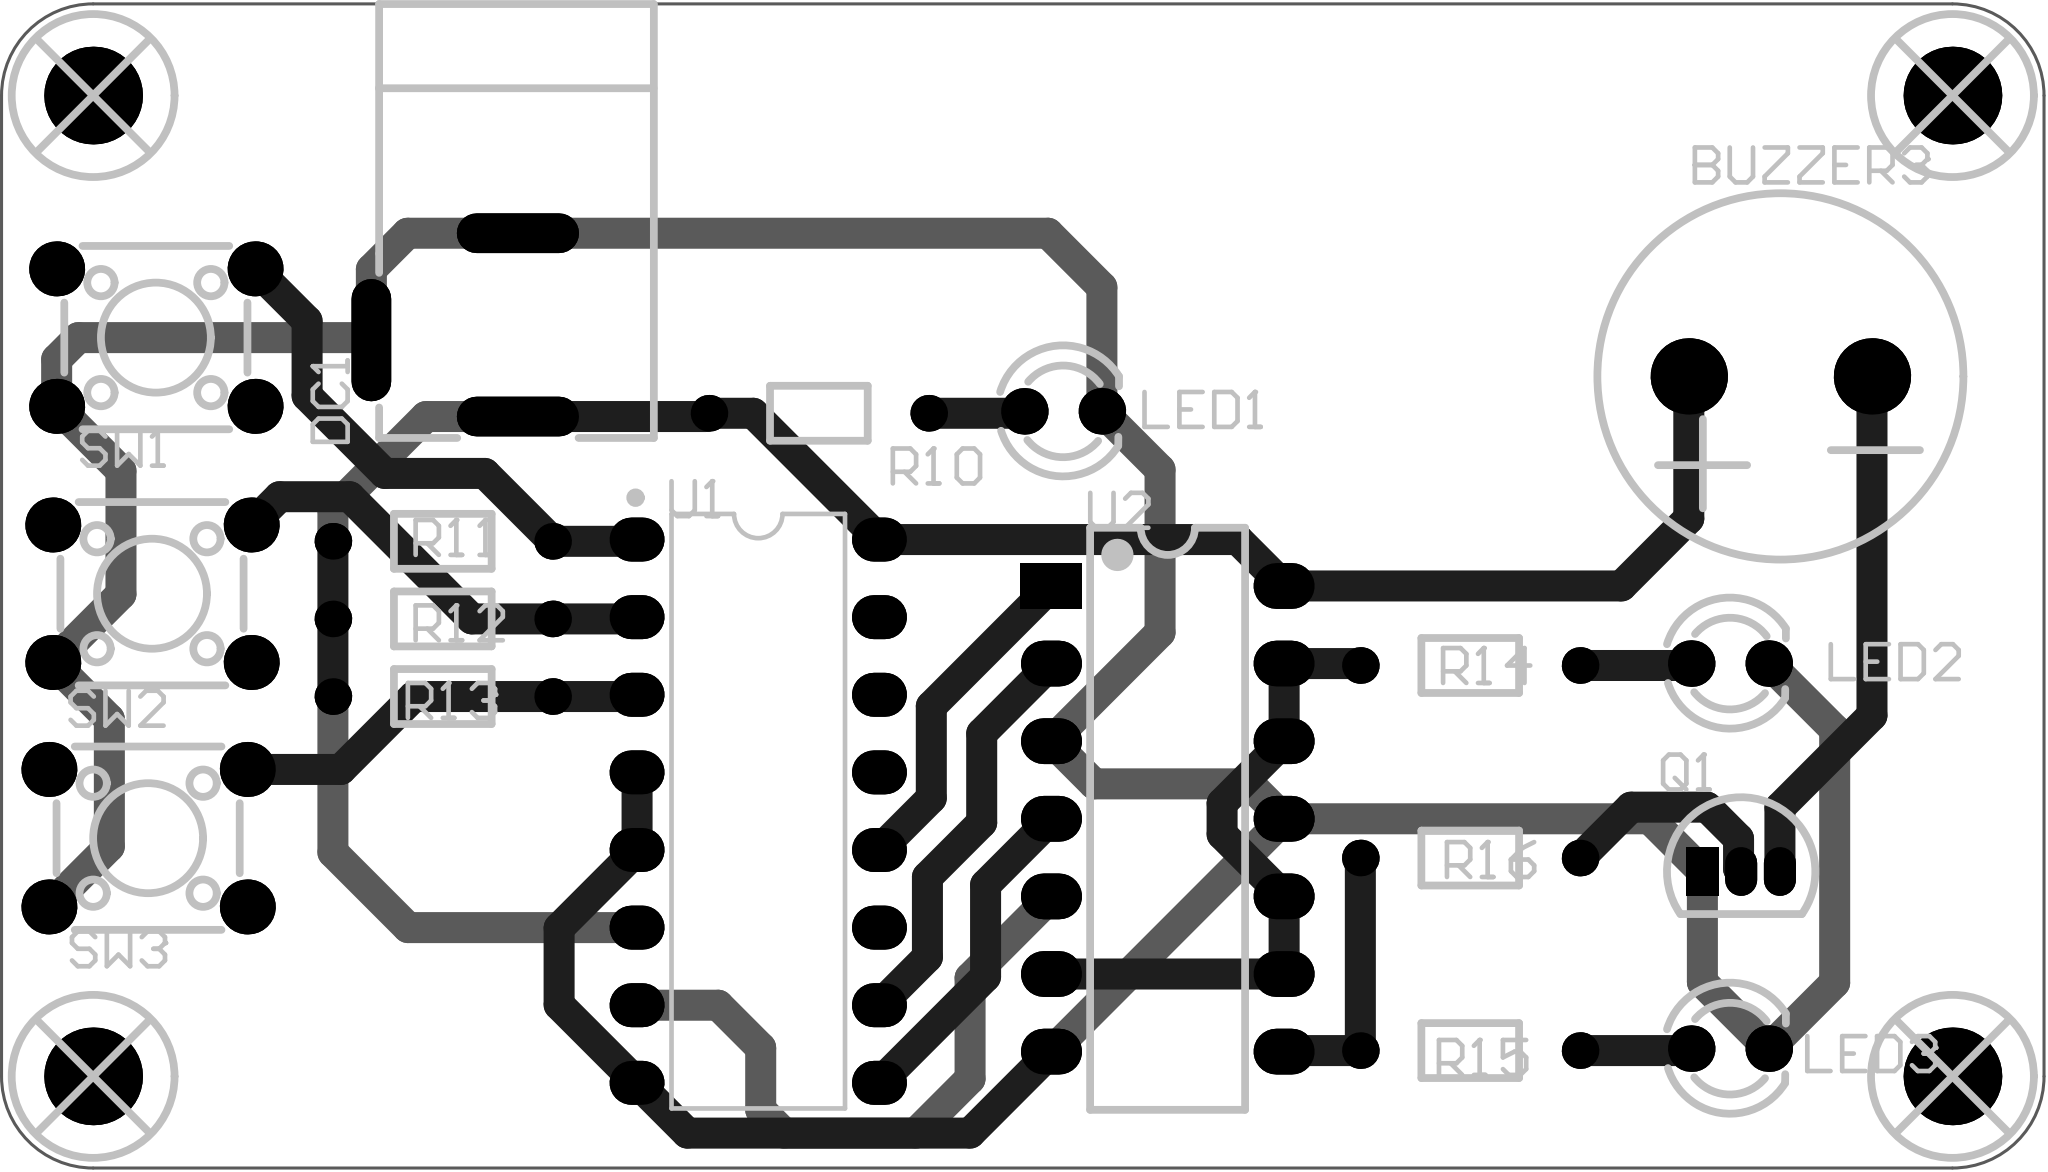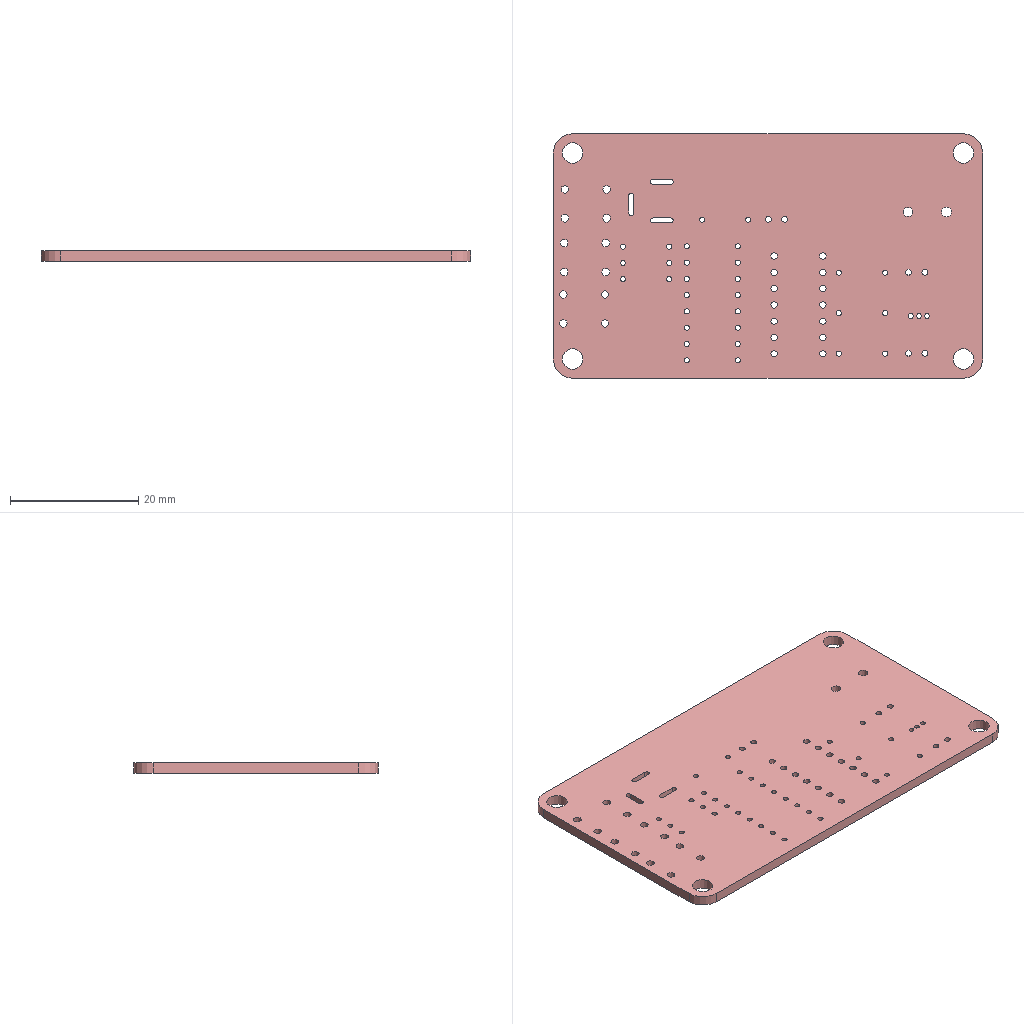Circuit board layout | Altium Designer | box 66.9 x 38.1 x 1.6 mm
Layer stack:
# Altium Designer layer stack of  (unit mm; dielectric type: 0 none, 1 core, 2 prepreg, 3 surface material)
index,name,kind,layer,copper_thickness_mm,dielectric_type,dielectric_thickness_mm,dielectric_material,dielectric_constant
0,Top Paste Mask Layer,other,,,,,,
1,Top Silkscreen Layer,other,,,,,,
2,Top Solder Mask Layer,dielectric,,,3,0.01,,3.3
3,Top Layer,copper,Top Layer,0.035,,,,
4,Dielectric1,dielectric,,,3,1.51,FR4,4.5
5,Bottom Layer,copper,Bottom Layer,0.035,,,,
6,Bottom Solder Mask Layer,dielectric,,,3,0.01,,3.3
7,Bottom Silkscreen Layer,other,,,,,,
8,Bottom Paste Mask Layer,other,,,,,,
# drill layer pairs: low layer,high layer
drill_pair,Top Layer,Bottom Layer
Part placement:
Designator,Comment,Layer,Footprint,Center-X(mm),Center-Y(mm),Rotation
LED2,,TopLayer,LED_TH-3mm,132.817,92.71,0
LED3,,TopLayer,LED_TH-3mm,132.817,80.107,0
Q1,SS8050BBU,TopLayer,TO-92-3_L4.8-W3.7-P1.27-L-1,133.183,85.905,0
SCREW1,,TopLayer,M3螺丝,79.2,79.2,0
SCREW2,,TopLayer,M3螺丝,140.104,79.2,0
SCREW3,,TopLayer,M3螺丝,79.2,111.3,0
SCREW4,,TopLayer,M3螺丝,140.104,111.3,0
R11,10kΩ,TopLayer,Res_1/8W,90.653,96.711,180
R12,10kΩ,TopLayer,Res_1/8W,90.653,94.171,180
R13,10kΩ,TopLayer,Res_1/8W,90.653,91.631,180
R14,510Ω,TopLayer,Res_1/8W,124.308,92.647,180
R15,510Ω,TopLayer,Res_1/8W,124.308,80.044,180
SW1,,TopLayer,SW-TH_4P-L6.0-W6.0-P4.50-LS6.5,81.255,103.378,180
SW2,,TopLayer,SW-TH_4P-L6.0-W6.0-P4.50-LS6.5,81.128,94.996,180
LED1,,TopLayer,LED_TH-3mm,110.973,100.965,0
R10,1kΩ,TopLayer,Res_1/8W,102.972,100.902,180
SW3,,TopLayer,SW-TH_4P-L6.0-W6.0-P4.50-LS6.5,81.001,86.995,180
U1,SN74HC138N(LX),TopLayer,PDIP-16_L19.3-W6.4-P2.54-LS7.94-BL,100.987,87.879,270
U2,SN74HC20N(LX),TopLayer,PDIP-14_L19.3-W6.5-P2.54-LS7.6-BL,114.402,87.63,270
BUZZER3,buzzer,TopLayer,BUZ-TH_BD12.0-P6.00-D0.9-RD,134.468,102.108,180
R16,10kΩ,TopLayer,Res_1/8W,124.308,86.346,0
DC1,,TopLayer,DC-2.0,90.714,103.795,90
Pad and via stacks:
# Altium Designer via and pad stacks of  (unit mm). Each distinct definition once, with the count of objects using it.
# via: kind,start_layer,end_layer,hole_mm,diameter_mm,mode(0 simple;1 top-mid-bottom;2 full stack),diameter_per_layer,count,example_net
# pad: kind,layer,hole_mm,hole_type(0 round;1 square;2 slot),plating,top_size,top_shape(1 round;2 rect;3 octagon;9 rounded rect),mid_size,bottom_size,mode,footprint,size_per_layer,count,example
pad,Multi-Layer,0.9144,0,plated,1.524x1.524,1,1.524x1.524,1.524x1.524,0,LED_TH-3mm,,6,LED2.1
pad,Multi-Layer,0.75,0,plated,1.05x1.6,1,1.05x1.6,1.05x1.6,0,TO-92-3_L4.8-W3.7-P1.27-L-1,,2,Q1.3
pad,Multi-Layer,0.75,0,plated,1.05x1.6,2,1.05x1.6,1.05x1.6,0,TO-92-3_L4.8-W3.7-P1.27-L-1,,1,Q1.1
pad,Multi-Layer,3.2,0,plated,3.2x3.2,1,3.2x3.2,3.2x3.2,0,M3\u00C2\u00DD\u00CB\u00BF,,4,SCREW1.1
pad,Multi-Layer,0.8001,0,plated,1.199x1.199,1,1.199x1.199,1.199x1.199,0,Res_1/8W,,14,R11.1
pad,Multi-Layer,1.2,0,plated,1.8x1.8,1,1.8x1.8,1.8x1.8,0,SW-TH_4P-L6.0-W6.0-P4.50-LS6.5,,12,SW1.1
pad,Multi-Layer,0.8,0,plated,1.44x1.8,1,1.44x1.8,1.44x1.8,0,PDIP-16_L19.3-W6.4-P2.54-LS7.94-BL,,16,U1.1
pad,Multi-Layer,1,0,plated,1.5x2,1,1.5x2,1.5x2,0,PDIP-14_L19.3-W6.5-P2.54-LS7.6-BL,,13,U2.8
pad,Multi-Layer,1,0,plated,1.5x2,2,1.5x2,1.5x2,0,PDIP-14_L19.3-W6.5-P2.54-LS7.6-BL,,1,U2.1
pad,Multi-Layer,1.5,0,plated,2.5x2.5,1,2.5x2.5,2.5x2.5,0,BUZ-TH_BD12.0-P6.00-D0.9-RD,,2,BUZZER3.1
pad,Multi-Layer,0.8001,2,plated,4x1.3,1,4x1.3,4x1.3,0,DC-2.0,,3,DC1.2